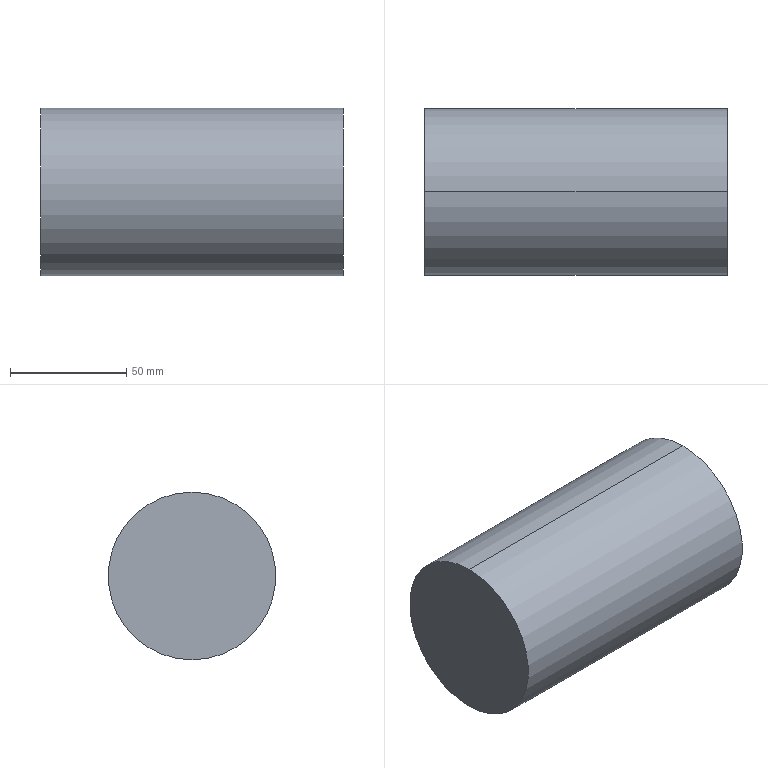Part | SolidWorks | features BaseBody 1 | 1 solid | 4 faces | box 130 x 72 x 72 mm | volume 529296 mm3 | cylinder 2 | plane 2 | commonest cylinder face diameters 72 x2
STEP:
#1=CARTESIAN_POINT('',(130.,0.,36.));
#2=VERTEX_POINT('',#1);
#3=CARTESIAN_POINT('',(130.,0.,-36.));
#4=VERTEX_POINT('',#3);
#5=CARTESIAN_POINT('',(130.,0.,0.));
#6=DIRECTION('',(-1.,0.,0.));
#7=DIRECTION('',(0.,0.,1.));
#8=AXIS2_PLACEMENT_3D('',#5,#6,#7);
#9=CIRCLE('',#8,36.);
#10=EDGE_CURVE('',#2,#4,#9,.T.);
#11=ORIENTED_EDGE('',*,*,#10,.T.);
#12=CARTESIAN_POINT('',(0.,0.,-36.));
#13=VERTEX_POINT('',#12);
#14=CARTESIAN_POINT('',(130.,0.,-36.));
#15=DIRECTION('',(-1.,0.,0.));
#16=VECTOR('',#15,1000.);
#17=LINE('',#14,#16);
#18=EDGE_CURVE('',#4,#13,#17,.T.);
#19=ORIENTED_EDGE('',*,*,#18,.T.);
#20=CARTESIAN_POINT('',(0.,0.,36.));
#21=VERTEX_POINT('',#20);
#22=CARTESIAN_POINT('',(0.,0.,0.));
#23=DIRECTION('',(1.,0.,0.));
#24=DIRECTION('',(0.,0.,1.));
#25=AXIS2_PLACEMENT_3D('',#22,#23,#24);
#26=CIRCLE('',#25,36.);
#27=EDGE_CURVE('',#13,#21,#26,.T.);
#28=ORIENTED_EDGE('',*,*,#27,.T.);
#29=CARTESIAN_POINT('',(130.,0.,36.));
#30=DIRECTION('',(-1.,0.,0.));
#31=VECTOR('',#30,1000.);
#32=LINE('',#29,#31);
#33=EDGE_CURVE('',#2,#21,#32,.T.);
#34=ORIENTED_EDGE('',*,*,#33,.F.);
#35=EDGE_LOOP('',(#11,#19,#28,#34));
#36=FACE_OUTER_BOUND('',#35,.T.);
#37=CARTESIAN_POINT('',(130.,0.,0.));
#38=DIRECTION('',(-1.,0.,0.));
#39=DIRECTION('',(0.,0.,1.));
#40=AXIS2_PLACEMENT_3D('',#37,#38,#39);
#41=CYLINDRICAL_SURFACE('',#40,36.);
#42=ADVANCED_FACE('',(#36),#41,.T.);
#43=ORIENTED_EDGE('',*,*,#18,.F.);
#44=CARTESIAN_POINT('',(130.,0.,0.));
#45=DIRECTION('',(-1.,0.,0.));
#46=DIRECTION('',(0.,0.,1.));
#47=AXIS2_PLACEMENT_3D('',#44,#45,#46);
#48=CIRCLE('',#47,36.);
#49=EDGE_CURVE('',#4,#2,#48,.T.);
#50=ORIENTED_EDGE('',*,*,#49,.T.);
#51=ORIENTED_EDGE('',*,*,#33,.T.);
#52=CARTESIAN_POINT('',(0.,0.,0.));
#53=DIRECTION('',(1.,0.,0.));
#54=DIRECTION('',(0.,0.,1.));
#55=AXIS2_PLACEMENT_3D('',#52,#53,#54);
#56=CIRCLE('',#55,36.);
#57=EDGE_CURVE('',#21,#13,#56,.T.);
#58=ORIENTED_EDGE('',*,*,#57,.T.);
#59=EDGE_LOOP('',(#43,#50,#51,#58));
#60=FACE_OUTER_BOUND('',#59,.T.);
#61=CARTESIAN_POINT('',(130.,0.,0.));
#62=DIRECTION('',(-1.,0.,0.));
#63=DIRECTION('',(0.,0.,1.));
#64=AXIS2_PLACEMENT_3D('',#61,#62,#63);
#65=CYLINDRICAL_SURFACE('',#64,36.);
#66=ADVANCED_FACE('',(#60),#65,.T.);
#67=ORIENTED_EDGE('',*,*,#57,.F.);
#68=ORIENTED_EDGE('',*,*,#27,.F.);
#69=EDGE_LOOP('',(#67,#68));
#70=FACE_OUTER_BOUND('',#69,.T.);
#71=CARTESIAN_POINT('',(0.,0.,0.));
#72=DIRECTION('',(1.,0.,0.));
#73=DIRECTION('',(0.,0.,-1.));
#74=AXIS2_PLACEMENT_3D('',#71,#72,#73);
#75=PLANE('',#74);
#76=ADVANCED_FACE('',(#70),#75,.F.);
#77=ORIENTED_EDGE('',*,*,#10,.F.);
#78=ORIENTED_EDGE('',*,*,#49,.F.);
#79=EDGE_LOOP('',(#77,#78));
#80=FACE_OUTER_BOUND('',#79,.T.);
#81=CARTESIAN_POINT('',(130.,0.,0.));
#82=DIRECTION('',(1.,0.,0.));
#83=DIRECTION('',(0.,0.,-1.));
#84=AXIS2_PLACEMENT_3D('',#81,#82,#83);
#85=PLANE('',#84);
#86=ADVANCED_FACE('',(#80),#85,.T.);
#87=CLOSED_SHELL('',(#42,#66,#76,#86));
#88=MANIFOLD_SOLID_BREP('',#87);
#89=CARTESIAN_POINT('',(0.,0.,0.));
#90=DIRECTION('',(0.,0.,1.));
#91=DIRECTION('',(1.,0.,0.));
#92=AXIS2_PLACEMENT_3D('',#89,#90,#91);
#93=(LENGTH_UNIT()NAMED_UNIT(*)SI_UNIT(.MILLI.,.METRE.));
#94=UNCERTAINTY_MEASURE_WITH_UNIT(LENGTH_MEASURE(0.00001),#93,'','');
#95=(NAMED_UNIT(*)PLANE_ANGLE_UNIT()SI_UNIT($,.RADIAN.));
#96=(NAMED_UNIT(*)SI_UNIT($,.STERADIAN.)SOLID_ANGLE_UNIT());
#97=(GEOMETRIC_REPRESENTATION_CONTEXT(3)GLOBAL_UNCERTAINTY_ASSIGNED_CONTEXT((#94))GLOBAL_UNIT_ASSIGNED_CONTEXT((#93,#95,#96))REPRESENTATION_CONTEXT('',''));
#98=ADVANCED_BREP_SHAPE_REPRESENTATION('',(#88,#92),#97);